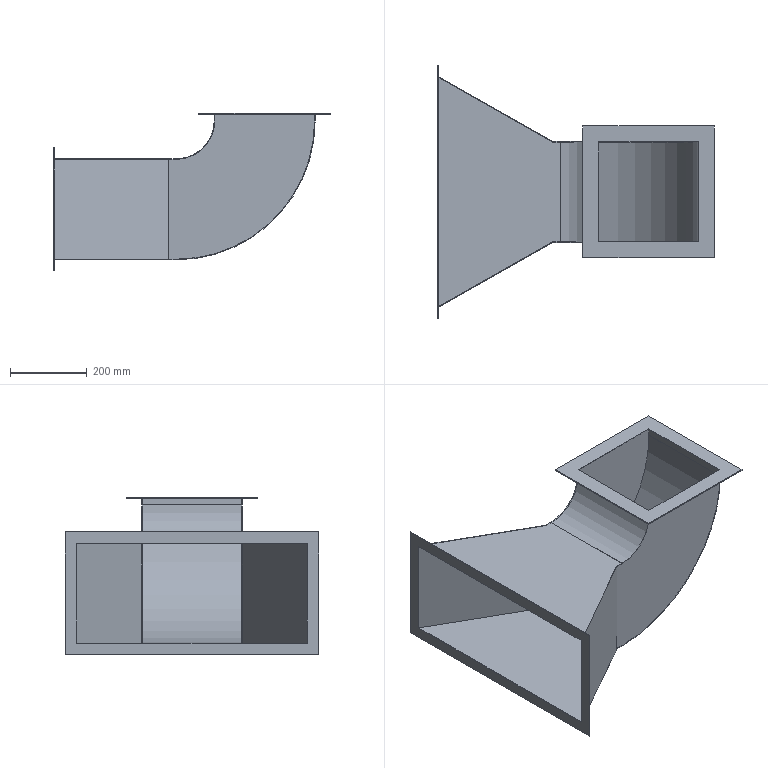Part | STEP file | Produce dryer line heating fan-OVEN-402 | 1 solid | 34 faces | box 721.5 x 660 x 410 mm | volume 1592936 mm3 | plane 30 | cylinder 4 | commonest cylinder face diameters 197 x1 200 x1 720 x1 723 x1
STEP:
#1=CARTESIAN_POINT('',(681.5,131.5,230.));
#2=VERTEX_POINT('',#1);
#3=CARTESIAN_POINT('',(681.5,131.5,247.));
#4=VERTEX_POINT('',#3);
#5=CARTESIAN_POINT('',(681.5,131.5,230.));
#6=DIRECTION('',(0.,0.,1.));
#7=VECTOR('',#6,1000.);
#8=LINE('',#5,#7);
#9=EDGE_CURVE('',#2,#4,#8,.T.);
#10=ORIENTED_EDGE('',*,*,#9,.T.);
#11=CARTESIAN_POINT('',(681.5,-131.5,247.));
#12=VERTEX_POINT('',#11);
#13=CARTESIAN_POINT('',(681.5,131.5,247.));
#14=DIRECTION('',(0.,1.,0.));
#15=VECTOR('',#14,1000.);
#16=LINE('',#13,#15);
#17=EDGE_CURVE('',#12,#4,#16,.T.);
#18=ORIENTED_EDGE('',*,*,#17,.F.);
#19=CARTESIAN_POINT('',(681.5,-131.5,230.));
#20=VERTEX_POINT('',#19);
#21=CARTESIAN_POINT('',(681.5,-131.5,230.));
#22=DIRECTION('',(0.,0.,1.));
#23=VECTOR('',#22,1000.);
#24=LINE('',#21,#23);
#25=EDGE_CURVE('',#20,#12,#24,.T.);
#26=ORIENTED_EDGE('',*,*,#25,.F.);
#27=CARTESIAN_POINT('',(681.5,130.,230.));
#28=DIRECTION('',(0.,1.,0.));
#29=VECTOR('',#28,1000.);
#30=LINE('',#27,#29);
#31=EDGE_CURVE('',#20,#2,#30,.T.);
#32=ORIENTED_EDGE('',*,*,#31,.T.);
#33=EDGE_LOOP('',(#10,#18,#26,#32));
#34=FACE_OUTER_BOUND('',#33,.T.);
#35=CARTESIAN_POINT('',(681.5,130.,230.));
#36=DIRECTION('',(1.,0.,0.));
#37=DIRECTION('',(0.,0.,-1.));
#38=AXIS2_PLACEMENT_3D('',#35,#36,#37);
#39=PLANE('',#38);
#40=ADVANCED_FACE('',(#34),#39,.T.);
#41=CARTESIAN_POINT('',(418.5,-131.5,230.));
#42=VERTEX_POINT('',#41);
#43=CARTESIAN_POINT('',(418.5,-131.5,247.));
#44=VERTEX_POINT('',#43);
#45=CARTESIAN_POINT('',(418.5,-131.5,230.));
#46=DIRECTION('',(0.,0.,1.));
#47=VECTOR('',#46,1000.);
#48=LINE('',#45,#47);
#49=EDGE_CURVE('',#42,#44,#48,.T.);
#50=ORIENTED_EDGE('',*,*,#49,.T.);
#51=CARTESIAN_POINT('',(418.5,131.5,247.));
#52=VERTEX_POINT('',#51);
#53=CARTESIAN_POINT('',(418.5,131.5,247.));
#54=DIRECTION('',(0.,-1.,0.));
#55=VECTOR('',#54,1000.);
#56=LINE('',#53,#55);
#57=EDGE_CURVE('',#52,#44,#56,.T.);
#58=ORIENTED_EDGE('',*,*,#57,.F.);
#59=CARTESIAN_POINT('',(418.5,131.5,230.));
#60=VERTEX_POINT('',#59);
#61=CARTESIAN_POINT('',(418.5,131.5,230.));
#62=DIRECTION('',(0.,0.,1.));
#63=VECTOR('',#62,1000.);
#64=LINE('',#61,#63);
#65=EDGE_CURVE('',#60,#52,#64,.T.);
#66=ORIENTED_EDGE('',*,*,#65,.F.);
#67=CARTESIAN_POINT('',(418.5,130.,230.));
#68=DIRECTION('',(0.,-1.,0.));
#69=VECTOR('',#68,1000.);
#70=LINE('',#67,#69);
#71=EDGE_CURVE('',#60,#42,#70,.T.);
#72=ORIENTED_EDGE('',*,*,#71,.T.);
#73=EDGE_LOOP('',(#50,#58,#66,#72));
#74=FACE_OUTER_BOUND('',#73,.T.);
#75=CARTESIAN_POINT('',(418.5,130.,230.));
#76=DIRECTION('',(-1.,0.,0.));
#77=DIRECTION('',(0.,0.,1.));
#78=AXIS2_PLACEMENT_3D('',#75,#76,#77);
#79=PLANE('',#78);
#80=ADVANCED_FACE('',(#74),#79,.T.);
#81=CARTESIAN_POINT('',(418.5,-131.5,247.));
#82=DIRECTION('',(1.,0.,0.));
#83=VECTOR('',#82,1000.);
#84=LINE('',#81,#83);
#85=EDGE_CURVE('',#44,#12,#84,.T.);
#86=ORIENTED_EDGE('',*,*,#85,.F.);
#87=ORIENTED_EDGE('',*,*,#49,.F.);
#88=CARTESIAN_POINT('',(320.,-131.5,131.5));
#89=VERTEX_POINT('',#88);
#90=CARTESIAN_POINT('',(320.,-131.5,230.));
#91=DIRECTION('',(0.,-1.,0.));
#92=DIRECTION('',(0.,0.,-1.));
#93=AXIS2_PLACEMENT_3D('',#90,#91,#92);
#94=CIRCLE('',#93,98.5);
#95=EDGE_CURVE('',#89,#42,#94,.T.);
#96=ORIENTED_EDGE('',*,*,#95,.F.);
#97=CARTESIAN_POINT('',(300.,-131.5,131.5));
#98=VERTEX_POINT('',#97);
#99=CARTESIAN_POINT('',(320.,-131.5,131.5));
#100=DIRECTION('',(-1.,0.,0.));
#101=VECTOR('',#100,1000.);
#102=LINE('',#99,#101);
#103=EDGE_CURVE('',#89,#98,#102,.T.);
#104=ORIENTED_EDGE('',*,*,#103,.T.);
#105=CARTESIAN_POINT('',(300.,-131.5,-131.5));
#106=VERTEX_POINT('',#105);
#107=CARTESIAN_POINT('',(300.,-131.5,130.));
#108=DIRECTION('',(0.,0.,-1.));
#109=VECTOR('',#108,1000.);
#110=LINE('',#107,#109);
#111=EDGE_CURVE('',#98,#106,#110,.T.);
#112=ORIENTED_EDGE('',*,*,#111,.T.);
#113=CARTESIAN_POINT('',(320.,-131.5,-131.5));
#114=VERTEX_POINT('',#113);
#115=CARTESIAN_POINT('',(320.,-131.5,-131.5));
#116=DIRECTION('',(-1.,0.,0.));
#117=VECTOR('',#116,1000.);
#118=LINE('',#115,#117);
#119=EDGE_CURVE('',#114,#106,#118,.T.);
#120=ORIENTED_EDGE('',*,*,#119,.F.);
#121=CARTESIAN_POINT('',(320.,-131.5,230.));
#122=DIRECTION('',(0.,-1.,0.));
#123=DIRECTION('',(0.,0.,-1.));
#124=AXIS2_PLACEMENT_3D('',#121,#122,#123);
#125=CIRCLE('',#124,361.5);
#126=EDGE_CURVE('',#114,#20,#125,.T.);
#127=ORIENTED_EDGE('',*,*,#126,.T.);
#128=ORIENTED_EDGE('',*,*,#25,.T.);
#129=EDGE_LOOP('',(#86,#87,#96,#104,#112,#120,#127,#128));
#130=FACE_OUTER_BOUND('',#129,.T.);
#131=CARTESIAN_POINT('',(320.,-131.5,130.));
#132=DIRECTION('',(0.,1.,0.));
#133=DIRECTION('',(0.,0.,1.));
#134=AXIS2_PLACEMENT_3D('',#131,#132,#133);
#135=PLANE('',#134);
#136=ADVANCED_FACE('',(#130),#135,.F.);
#137=CARTESIAN_POINT('',(418.5,131.5,247.));
#138=DIRECTION('',(-1.,0.,0.));
#139=VECTOR('',#138,1000.);
#140=LINE('',#137,#139);
#141=EDGE_CURVE('',#4,#52,#140,.T.);
#142=ORIENTED_EDGE('',*,*,#141,.F.);
#143=ORIENTED_EDGE('',*,*,#9,.F.);
#144=CARTESIAN_POINT('',(320.,131.5,-131.5));
#145=VERTEX_POINT('',#144);
#146=CARTESIAN_POINT('',(320.,131.5,230.));
#147=DIRECTION('',(0.,-1.,0.));
#148=DIRECTION('',(0.,0.,1.));
#149=AXIS2_PLACEMENT_3D('',#146,#147,#148);
#150=CIRCLE('',#149,361.5);
#151=EDGE_CURVE('',#145,#2,#150,.T.);
#152=ORIENTED_EDGE('',*,*,#151,.F.);
#153=CARTESIAN_POINT('',(300.,131.5,-131.5));
#154=VERTEX_POINT('',#153);
#155=CARTESIAN_POINT('',(320.,131.5,-131.5));
#156=DIRECTION('',(-1.,0.,0.));
#157=VECTOR('',#156,1000.);
#158=LINE('',#155,#157);
#159=EDGE_CURVE('',#145,#154,#158,.T.);
#160=ORIENTED_EDGE('',*,*,#159,.T.);
#161=CARTESIAN_POINT('',(300.,131.5,131.5));
#162=VERTEX_POINT('',#161);
#163=CARTESIAN_POINT('',(300.,131.5,130.));
#164=DIRECTION('',(0.,0.,1.));
#165=VECTOR('',#164,1000.);
#166=LINE('',#163,#165);
#167=EDGE_CURVE('',#154,#162,#166,.T.);
#168=ORIENTED_EDGE('',*,*,#167,.T.);
#169=CARTESIAN_POINT('',(320.,131.5,131.5));
#170=VERTEX_POINT('',#169);
#171=CARTESIAN_POINT('',(320.,131.5,131.5));
#172=DIRECTION('',(-1.,0.,0.));
#173=VECTOR('',#172,1000.);
#174=LINE('',#171,#173);
#175=EDGE_CURVE('',#170,#162,#174,.T.);
#176=ORIENTED_EDGE('',*,*,#175,.F.);
#177=CARTESIAN_POINT('',(320.,131.5,230.));
#178=DIRECTION('',(0.,-1.,0.));
#179=DIRECTION('',(0.,0.,1.));
#180=AXIS2_PLACEMENT_3D('',#177,#178,#179);
#181=CIRCLE('',#180,98.5);
#182=EDGE_CURVE('',#170,#60,#181,.T.);
#183=ORIENTED_EDGE('',*,*,#182,.T.);
#184=ORIENTED_EDGE('',*,*,#65,.T.);
#185=EDGE_LOOP('',(#142,#143,#152,#160,#168,#176,#183,#184));
#186=FACE_OUTER_BOUND('',#185,.T.);
#187=CARTESIAN_POINT('',(320.,131.5,130.));
#188=DIRECTION('',(0.,-1.,0.));
#189=DIRECTION('',(0.,0.,-1.));
#190=AXIS2_PLACEMENT_3D('',#187,#188,#189);
#191=PLANE('',#190);
#192=ADVANCED_FACE('',(#186),#191,.F.);
#193=ORIENTED_EDGE('',*,*,#167,.F.);
#194=CARTESIAN_POINT('',(300.,131.724,-131.5));
#195=VERTEX_POINT('',#194);
#196=CARTESIAN_POINT('',(300.,130.,-131.5));
#197=DIRECTION('',(0.,1.,0.));
#198=VECTOR('',#197,1000.);
#199=LINE('',#196,#198);
#200=EDGE_CURVE('',#154,#195,#199,.T.);
#201=ORIENTED_EDGE('',*,*,#200,.T.);
#202=CARTESIAN_POINT('',(300.,131.724,131.5));
#203=VERTEX_POINT('',#202);
#204=CARTESIAN_POINT('',(300.,131.724,130.));
#205=DIRECTION('',(0.,0.,1.));
#206=VECTOR('',#205,1000.);
#207=LINE('',#204,#206);
#208=EDGE_CURVE('',#195,#203,#207,.T.);
#209=ORIENTED_EDGE('',*,*,#208,.T.);
#210=CARTESIAN_POINT('',(300.,-130.,131.5));
#211=DIRECTION('',(0.,-1.,0.));
#212=VECTOR('',#211,1000.);
#213=LINE('',#210,#212);
#214=EDGE_CURVE('',#203,#162,#213,.T.);
#215=ORIENTED_EDGE('',*,*,#214,.T.);
#216=EDGE_LOOP('',(#193,#201,#209,#215));
#217=FACE_OUTER_BOUND('',#216,.T.);
#218=CARTESIAN_POINT('',(300.,-130.,130.));
#219=DIRECTION('',(1.,0.,0.));
#220=DIRECTION('',(0.,0.,-1.));
#221=AXIS2_PLACEMENT_3D('',#218,#219,#220);
#222=PLANE('',#221);
#223=ADVANCED_FACE('',(#217),#222,.T.);
#224=CARTESIAN_POINT('',(3.,330.,160.));
#225=VERTEX_POINT('',#224);
#226=CARTESIAN_POINT('',(3.,-330.,160.));
#227=VERTEX_POINT('',#226);
#228=CARTESIAN_POINT('',(3.,330.,160.));
#229=DIRECTION('',(0.,-1.,0.));
#230=VECTOR('',#229,1000.);
#231=LINE('',#228,#230);
#232=EDGE_CURVE('',#225,#227,#231,.T.);
#233=ORIENTED_EDGE('',*,*,#232,.T.);
#234=CARTESIAN_POINT('',(3.,-330.,-160.));
#235=VERTEX_POINT('',#234);
#236=CARTESIAN_POINT('',(3.,-330.,160.));
#237=DIRECTION('',(0.,0.,-1.));
#238=VECTOR('',#237,1000.);
#239=LINE('',#236,#238);
#240=EDGE_CURVE('',#227,#235,#239,.T.);
#241=ORIENTED_EDGE('',*,*,#240,.T.);
#242=CARTESIAN_POINT('',(3.,330.,-160.));
#243=VERTEX_POINT('',#242);
#244=CARTESIAN_POINT('',(3.,330.,-160.));
#245=DIRECTION('',(0.,1.,0.));
#246=VECTOR('',#245,1000.);
#247=LINE('',#244,#246);
#248=EDGE_CURVE('',#235,#243,#247,.T.);
#249=ORIENTED_EDGE('',*,*,#248,.T.);
#250=CARTESIAN_POINT('',(3.,330.,160.));
#251=DIRECTION('',(0.,0.,1.));
#252=VECTOR('',#251,1000.);
#253=LINE('',#250,#252);
#254=EDGE_CURVE('',#243,#225,#253,.T.);
#255=ORIENTED_EDGE('',*,*,#254,.T.);
#256=EDGE_LOOP('',(#233,#241,#249,#255));
#257=FACE_OUTER_BOUND('',#256,.T.);
#258=CARTESIAN_POINT('',(3.,300.024,-131.5));
#259=VERTEX_POINT('',#258);
#260=CARTESIAN_POINT('',(3.,-300.024,-131.5));
#261=VERTEX_POINT('',#260);
#262=CARTESIAN_POINT('',(3.,-330.,-131.5));
#263=DIRECTION('',(0.,-1.,0.));
#264=VECTOR('',#263,1000.);
#265=LINE('',#262,#264);
#266=EDGE_CURVE('',#259,#261,#265,.T.);
#267=ORIENTED_EDGE('',*,*,#266,.T.);
#268=CARTESIAN_POINT('',(3.,-300.024,131.5));
#269=VERTEX_POINT('',#268);
#270=CARTESIAN_POINT('',(3.,-300.024,160.));
#271=DIRECTION('',(0.,0.,1.));
#272=VECTOR('',#271,1000.);
#273=LINE('',#270,#272);
#274=EDGE_CURVE('',#261,#269,#273,.T.);
#275=ORIENTED_EDGE('',*,*,#274,.T.);
#276=CARTESIAN_POINT('',(3.,300.024,131.5));
#277=VERTEX_POINT('',#276);
#278=CARTESIAN_POINT('',(3.,-330.,131.5));
#279=DIRECTION('',(0.,1.,0.));
#280=VECTOR('',#279,1000.);
#281=LINE('',#278,#280);
#282=EDGE_CURVE('',#269,#277,#281,.T.);
#283=ORIENTED_EDGE('',*,*,#282,.T.);
#284=CARTESIAN_POINT('',(3.,300.024,160.));
#285=DIRECTION('',(0.,0.,-1.));
#286=VECTOR('',#285,1000.);
#287=LINE('',#284,#286);
#288=EDGE_CURVE('',#277,#259,#287,.T.);
#289=ORIENTED_EDGE('',*,*,#288,.T.);
#290=EDGE_LOOP('',(#267,#275,#283,#289));
#291=FACE_BOUND('',#290,.T.);
#292=CARTESIAN_POINT('',(3.,-330.,160.));
#293=DIRECTION('',(1.,0.,0.));
#294=DIRECTION('',(0.,0.,-1.));
#295=AXIS2_PLACEMENT_3D('',#292,#293,#294);
#296=PLANE('',#295);
#297=ADVANCED_FACE('',(#257,#291),#296,.T.);
#298=CARTESIAN_POINT('',(0.,300.,130.));
#299=VERTEX_POINT('',#298);
#300=CARTESIAN_POINT('',(0.,-300.,130.));
#301=VERTEX_POINT('',#300);
#302=CARTESIAN_POINT('',(0.,300.,130.));
#303=DIRECTION('',(0.,-1.,0.));
#304=VECTOR('',#303,1000.);
#305=LINE('',#302,#304);
#306=EDGE_CURVE('',#299,#301,#305,.T.);
#307=ORIENTED_EDGE('',*,*,#306,.T.);
#308=CARTESIAN_POINT('',(0.,-300.,-130.));
#309=VERTEX_POINT('',#308);
#310=CARTESIAN_POINT('',(0.,-300.,130.));
#311=CARTESIAN_POINT('',(0.,-300.,43.333));
#312=CARTESIAN_POINT('',(0.,-300.,-43.333));
#313=CARTESIAN_POINT('',(0.,-300.,-130.));
#314=B_SPLINE_CURVE_WITH_KNOTS('',3,(#310,#311,#312,#313),.UNSPECIFIED.,.F.,.F.,(4,4),(0.,1.),.UNSPECIFIED.);
#315=EDGE_CURVE('',#301,#309,#314,.T.);
#316=ORIENTED_EDGE('',*,*,#315,.T.);
#317=CARTESIAN_POINT('',(0.,300.,-130.));
#318=VERTEX_POINT('',#317);
#319=CARTESIAN_POINT('',(0.,300.,-130.));
#320=DIRECTION('',(0.,1.,0.));
#321=VECTOR('',#320,1000.);
#322=LINE('',#319,#321);
#323=EDGE_CURVE('',#309,#318,#322,.T.);
#324=ORIENTED_EDGE('',*,*,#323,.T.);
#325=CARTESIAN_POINT('',(0.,300.,-130.));
#326=CARTESIAN_POINT('',(0.,300.,-43.333));
#327=CARTESIAN_POINT('',(0.,300.,43.333));
#328=CARTESIAN_POINT('',(0.,300.,130.));
#329=B_SPLINE_CURVE_WITH_KNOTS('',3,(#325,#326,#327,#328),.UNSPECIFIED.,.F.,.F.,(4,4),(0.,1.),.UNSPECIFIED.);
#330=EDGE_CURVE('',#318,#299,#329,.T.);
#331=ORIENTED_EDGE('',*,*,#330,.T.);
#332=EDGE_LOOP('',(#307,#316,#324,#331));
#333=FACE_BOUND('',#332,.T.);
#334=CARTESIAN_POINT('',(0.,330.,160.));
#335=VERTEX_POINT('',#334);
#336=CARTESIAN_POINT('',(0.,-330.,160.));
#337=VERTEX_POINT('',#336);
#338=CARTESIAN_POINT('',(0.,330.,160.));
#339=DIRECTION('',(0.,-1.,0.));
#340=VECTOR('',#339,1000.);
#341=LINE('',#338,#340);
#342=EDGE_CURVE('',#335,#337,#341,.T.);
#343=ORIENTED_EDGE('',*,*,#342,.F.);
#344=CARTESIAN_POINT('',(0.,330.,-160.));
#345=VERTEX_POINT('',#344);
#346=CARTESIAN_POINT('',(0.,330.,160.));
#347=DIRECTION('',(0.,0.,1.));
#348=VECTOR('',#347,1000.);
#349=LINE('',#346,#348);
#350=EDGE_CURVE('',#345,#335,#349,.T.);
#351=ORIENTED_EDGE('',*,*,#350,.F.);
#352=CARTESIAN_POINT('',(0.,-330.,-160.));
#353=VERTEX_POINT('',#352);
#354=CARTESIAN_POINT('',(0.,330.,-160.));
#355=DIRECTION('',(0.,1.,0.));
#356=VECTOR('',#355,1000.);
#357=LINE('',#354,#356);
#358=EDGE_CURVE('',#353,#345,#357,.T.);
#359=ORIENTED_EDGE('',*,*,#358,.F.);
#360=CARTESIAN_POINT('',(0.,-330.,160.));
#361=DIRECTION('',(0.,0.,-1.));
#362=VECTOR('',#361,1000.);
#363=LINE('',#360,#362);
#364=EDGE_CURVE('',#337,#353,#363,.T.);
#365=ORIENTED_EDGE('',*,*,#364,.F.);
#366=EDGE_LOOP('',(#343,#351,#359,#365));
#367=FACE_OUTER_BOUND('',#366,.T.);
#368=CARTESIAN_POINT('',(0.,-330.,160.));
#369=DIRECTION('',(1.,0.,0.));
#370=DIRECTION('',(0.,0.,-1.));
#371=AXIS2_PLACEMENT_3D('',#368,#369,#370);
#372=PLANE('',#371);
#373=ADVANCED_FACE('',(#333,#367),#372,.F.);
#374=ORIENTED_EDGE('',*,*,#342,.T.);
#375=CARTESIAN_POINT('',(3.,-330.,160.));
#376=DIRECTION('',(-1.,0.,0.));
#377=VECTOR('',#376,1000.);
#378=LINE('',#375,#377);
#379=EDGE_CURVE('',#227,#337,#378,.T.);
#380=ORIENTED_EDGE('',*,*,#379,.F.);
#381=ORIENTED_EDGE('',*,*,#232,.F.);
#382=CARTESIAN_POINT('',(3.,330.,160.));
#383=DIRECTION('',(-1.,0.,0.));
#384=VECTOR('',#383,1000.);
#385=LINE('',#382,#384);
#386=EDGE_CURVE('',#225,#335,#385,.T.);
#387=ORIENTED_EDGE('',*,*,#386,.T.);
#388=EDGE_LOOP('',(#374,#380,#381,#387));
#389=FACE_OUTER_BOUND('',#388,.T.);
#390=CARTESIAN_POINT('',(3.,330.,160.));
#391=DIRECTION('',(0.,0.,-1.));
#392=DIRECTION('',(0.,1.,0.));
#393=AXIS2_PLACEMENT_3D('',#390,#391,#392);
#394=PLANE('',#393);
#395=ADVANCED_FACE('',(#389),#394,.F.);
#396=ORIENTED_EDGE('',*,*,#364,.T.);
#397=CARTESIAN_POINT('',(3.,-330.,-160.));
#398=DIRECTION('',(-1.,0.,0.));
#399=VECTOR('',#398,1000.);
#400=LINE('',#397,#399);
#401=EDGE_CURVE('',#235,#353,#400,.T.);
#402=ORIENTED_EDGE('',*,*,#401,.F.);
#403=ORIENTED_EDGE('',*,*,#240,.F.);
#404=ORIENTED_EDGE('',*,*,#379,.T.);
#405=EDGE_LOOP('',(#396,#402,#403,#404));
#406=FACE_OUTER_BOUND('',#405,.T.);
#407=CARTESIAN_POINT('',(3.,-330.,160.));
#408=DIRECTION('',(0.,1.,0.));
#409=DIRECTION('',(0.,0.,1.));
#410=AXIS2_PLACEMENT_3D('',#407,#408,#409);
#411=PLANE('',#410);
#412=ADVANCED_FACE('',(#406),#411,.F.);
#413=ORIENTED_EDGE('',*,*,#358,.T.);
#414=CARTESIAN_POINT('',(3.,330.,-160.));
#415=DIRECTION('',(-1.,0.,0.));
#416=VECTOR('',#415,1000.);
#417=LINE('',#414,#416);
#418=EDGE_CURVE('',#243,#345,#417,.T.);
#419=ORIENTED_EDGE('',*,*,#418,.F.);
#420=ORIENTED_EDGE('',*,*,#248,.F.);
#421=ORIENTED_EDGE('',*,*,#401,.T.);
#422=EDGE_LOOP('',(#413,#419,#420,#421));
#423=FACE_OUTER_BOUND('',#422,.T.);
#424=CARTESIAN_POINT('',(3.,330.,-160.));
#425=DIRECTION('',(0.,0.,1.));
#426=DIRECTION('',(0.,-1.,0.));
#427=AXIS2_PLACEMENT_3D('',#424,#425,#426);
#428=PLANE('',#427);
#429=ADVANCED_FACE('',(#423),#428,.F.);
#430=ORIENTED_EDGE('',*,*,#350,.T.);
#431=ORIENTED_EDGE('',*,*,#386,.F.);
#432=ORIENTED_EDGE('',*,*,#254,.F.);
#433=ORIENTED_EDGE('',*,*,#418,.T.);
#434=EDGE_LOOP('',(#430,#431,#432,#433));
#435=FACE_OUTER_BOUND('',#434,.T.);
#436=CARTESIAN_POINT('',(3.,330.,160.));
#437=DIRECTION('',(0.,-1.,0.));
#438=DIRECTION('',(0.,0.,-1.));
#439=AXIS2_PLACEMENT_3D('',#436,#437,#438);
#440=PLANE('',#439);
#441=ADVANCED_FACE('',(#435),#440,.F.);
#442=CARTESIAN_POINT('',(300.,-130.,130.));
#443=VERTEX_POINT('',#442);
#444=CARTESIAN_POINT('',(0.,-300.,130.));
#445=DIRECTION('',(0.87,0.493,0.));
#446=VECTOR('',#445,1000.);
#447=LINE('',#444,#446);
#448=EDGE_CURVE('',#301,#443,#447,.T.);
#449=ORIENTED_EDGE('',*,*,#448,.F.);
#450=ORIENTED_EDGE('',*,*,#306,.F.);
#451=CARTESIAN_POINT('',(300.,130.,130.));
#452=VERTEX_POINT('',#451);
#453=CARTESIAN_POINT('',(0.,300.,130.));
#454=DIRECTION('',(0.87,-0.493,0.));
#455=VECTOR('',#454,1000.);
#456=LINE('',#453,#455);
#457=EDGE_CURVE('',#299,#452,#456,.T.);
#458=ORIENTED_EDGE('',*,*,#457,.T.);
#459=CARTESIAN_POINT('',(320.,130.,130.));
#460=VERTEX_POINT('',#459);
#461=CARTESIAN_POINT('',(320.,130.,130.));
#462=DIRECTION('',(-1.,0.,0.));
#463=VECTOR('',#462,1000.);
#464=LINE('',#461,#463);
#465=EDGE_CURVE('',#460,#452,#464,.T.);
#466=ORIENTED_EDGE('',*,*,#465,.F.);
#467=CARTESIAN_POINT('',(320.,-130.,130.));
#468=VERTEX_POINT('',#467);
#469=CARTESIAN_POINT('',(320.,130.,130.));
#470=DIRECTION('',(0.,-1.,0.));
#471=VECTOR('',#470,1000.);
#472=LINE('',#469,#471);
#473=EDGE_CURVE('',#460,#468,#472,.T.);
#474=ORIENTED_EDGE('',*,*,#473,.T.);
#475=CARTESIAN_POINT('',(320.,-130.,130.));
#476=DIRECTION('',(-1.,0.,0.));
#477=VECTOR('',#476,1000.);
#478=LINE('',#475,#477);
#479=EDGE_CURVE('',#468,#443,#478,.T.);
#480=ORIENTED_EDGE('',*,*,#479,.T.);
#481=EDGE_LOOP('',(#449,#450,#458,#466,#474,#480));
#482=FACE_OUTER_BOUND('',#481,.T.);
#483=CARTESIAN_POINT('',(3.,300.,130.));
#484=DIRECTION('',(0.,0.,-1.));
#485=DIRECTION('',(-1.,0.,0.));
#486=AXIS2_PLACEMENT_3D('',#483,#484,#485);
#487=PLANE('',#486);
#488=ADVANCED_FACE('',(#482),#487,.T.);
#489=CARTESIAN_POINT('',(300.,-130.,-130.));
#490=VERTEX_POINT('',#489);
#491=CARTESIAN_POINT('',(0.,-300.,-130.));
#492=DIRECTION('',(0.87,0.493,0.));
#493=VECTOR('',#492,1000.);
#494=LINE('',#491,#493);
#495=EDGE_CURVE('',#309,#490,#494,.T.);
#496=ORIENTED_EDGE('',*,*,#495,.T.);
#497=CARTESIAN_POINT('',(320.,-130.,-130.));
#498=VERTEX_POINT('',#497);
#499=CARTESIAN_POINT('',(320.,-130.,-130.));
#500=DIRECTION('',(-1.,0.,0.));
#501=VECTOR('',#500,1000.);
#502=LINE('',#499,#501);
#503=EDGE_CURVE('',#498,#490,#502,.T.);
#504=ORIENTED_EDGE('',*,*,#503,.F.);
#505=CARTESIAN_POINT('',(320.,130.,-130.));
#506=VERTEX_POINT('',#505);
#507=CARTESIAN_POINT('',(320.,130.,-130.));
#508=DIRECTION('',(0.,1.,0.));
#509=VECTOR('',#508,1000.);
#510=LINE('',#507,#509);
#511=EDGE_CURVE('',#498,#506,#510,.T.);
#512=ORIENTED_EDGE('',*,*,#511,.T.);
#513=CARTESIAN_POINT('',(300.,130.,-130.));
#514=VERTEX_POINT('',#513);
#515=CARTESIAN_POINT('',(320.,130.,-130.));
#516=DIRECTION('',(-1.,0.,0.));
#517=VECTOR('',#516,1000.);
#518=LINE('',#515,#517);
#519=EDGE_CURVE('',#506,#514,#518,.T.);
#520=ORIENTED_EDGE('',*,*,#519,.T.);
#521=CARTESIAN_POINT('',(0.,300.,-130.));
#522=DIRECTION('',(0.87,-0.493,0.));
#523=VECTOR('',#522,1000.);
#524=LINE('',#521,#523);
#525=EDGE_CURVE('',#318,#514,#524,.T.);
#526=ORIENTED_EDGE('',*,*,#525,.F.);
#527=ORIENTED_EDGE('',*,*,#323,.F.);
#528=EDGE_LOOP('',(#496,#504,#512,#520,#526,#527));
#529=FACE_OUTER_BOUND('',#528,.T.);
#530=CARTESIAN_POINT('',(3.,300.,-130.));
#531=DIRECTION('',(0.,0.,1.));
#532=DIRECTION('',(0.,-1.,0.));
#533=AXIS2_PLACEMENT_3D('',#530,#531,#532);
#534=PLANE('',#533);
#535=ADVANCED_FACE('',(#529),#534,.T.);
#536=ORIENTED_EDGE('',*,*,#111,.F.);
#537=CARTESIAN_POINT('',(300.,-131.724,131.5));
#538=VERTEX_POINT('',#537);
#539=CARTESIAN_POINT('',(300.,-130.,131.5));
#540=DIRECTION('',(0.,-1.,0.));
#541=VECTOR('',#540,1000.);
#542=LINE('',#539,#541);
#543=EDGE_CURVE('',#98,#538,#542,.T.);
#544=ORIENTED_EDGE('',*,*,#543,.T.);
#545=CARTESIAN_POINT('',(300.,-131.724,-131.5));
#546=VERTEX_POINT('',#545);
#547=CARTESIAN_POINT('',(300.,-131.724,-130.));
#548=DIRECTION('',(0.,0.,-1.));
#549=VECTOR('',#548,1000.);
#550=LINE('',#547,#549);
#551=EDGE_CURVE('',#538,#546,#550,.T.);
#552=ORIENTED_EDGE('',*,*,#551,.T.);
#553=CARTESIAN_POINT('',(300.,130.,-131.5));
#554=DIRECTION('',(0.,1.,0.));
#555=VECTOR('',#554,1000.);
#556=LINE('',#553,#555);
#557=EDGE_CURVE('',#546,#106,#556,.T.);
#558=ORIENTED_EDGE('',*,*,#557,.T.);
#559=EDGE_LOOP('',(#536,#544,#552,#558));
#560=FACE_OUTER_BOUND('',#559,.T.);
#561=CARTESIAN_POINT('',(300.,-130.,130.));
#562=DIRECTION('',(1.,0.,0.));
#563=DIRECTION('',(0.,0.,-1.));
#564=AXIS2_PLACEMENT_3D('',#561,#562,#563);
#565=PLANE('',#564);
#566=ADVANCED_FACE('',(#560),#565,.T.);
#567=ORIENTED_EDGE('',*,*,#274,.F.);
#568=CARTESIAN_POINT('',(300.74,-131.305,-131.5));
#569=DIRECTION('',(0.87,0.493,0.));
#570=VECTOR('',#569,1000.);
#571=LINE('',#568,#570);
#572=EDGE_CURVE('',#261,#546,#571,.T.);
#573=ORIENTED_EDGE('',*,*,#572,.T.);
#574=ORIENTED_EDGE('',*,*,#551,.F.);
#575=CARTESIAN_POINT('',(300.74,-131.305,131.5));
#576=DIRECTION('',(0.87,0.493,0.));
#577=VECTOR('',#576,1000.);
#578=LINE('',#575,#577);
#579=EDGE_CURVE('',#269,#538,#578,.T.);
#580=ORIENTED_EDGE('',*,*,#579,.F.);
#581=EDGE_LOOP('',(#567,#573,#574,#580));
#582=FACE_OUTER_BOUND('',#581,.T.);
#583=CARTESIAN_POINT('',(300.74,-131.305,-130.));
#584=DIRECTION('',(-0.493,0.87,0.));
#585=DIRECTION('',(-0.87,-0.493,0.));
#586=AXIS2_PLACEMENT_3D('',#583,#584,#585);
#587=PLANE('',#586);
#588=ADVANCED_FACE('',(#582),#587,.F.);
#589=ORIENTED_EDGE('',*,*,#282,.F.);
#590=ORIENTED_EDGE('',*,*,#579,.T.);
#591=ORIENTED_EDGE('',*,*,#543,.F.);
#592=ORIENTED_EDGE('',*,*,#103,.F.);
#593=CARTESIAN_POINT('',(320.,0.,131.5));
#594=DIRECTION('',(0.,-1.,0.));
#595=VECTOR('',#594,1000.);
#596=LINE('',#593,#595);
#597=EDGE_CURVE('',#170,#89,#596,.T.);
#598=ORIENTED_EDGE('',*,*,#597,.F.);
#599=ORIENTED_EDGE('',*,*,#175,.T.);
#600=ORIENTED_EDGE('',*,*,#214,.F.);
#601=CARTESIAN_POINT('',(300.74,131.305,131.5));
#602=DIRECTION('',(0.87,-0.493,0.));
#603=VECTOR('',#602,1000.);
#604=LINE('',#601,#603);
#605=EDGE_CURVE('',#277,#203,#604,.T.);
#606=ORIENTED_EDGE('',*,*,#605,.F.);
#607=EDGE_LOOP('',(#589,#590,#591,#592,#598,#599,#600,#606));
#608=FACE_OUTER_BOUND('',#607,.T.);
#609=CARTESIAN_POINT('',(300.,-130.,131.5));
#610=DIRECTION('',(0.,0.,-1.));
#611=DIRECTION('',(-1.,0.,0.));
#612=AXIS2_PLACEMENT_3D('',#609,#610,#611);
#613=PLANE('',#612);
#614=ADVANCED_FACE('',(#608),#613,.F.);
#615=ORIENTED_EDGE('',*,*,#266,.F.);
#616=CARTESIAN_POINT('',(300.74,131.305,-131.5));
#617=DIRECTION('',(0.87,-0.493,0.));
#618=VECTOR('',#617,1000.);
#619=LINE('',#616,#618);
#620=EDGE_CURVE('',#259,#195,#619,.T.);
#621=ORIENTED_EDGE('',*,*,#620,.T.);
#622=ORIENTED_EDGE('',*,*,#200,.F.);
#623=ORIENTED_EDGE('',*,*,#159,.F.);
#624=CARTESIAN_POINT('',(320.,0.,-131.5));
#625=DIRECTION('',(0.,1.,0.));
#626=VECTOR('',#625,1000.);
#627=LINE('',#624,#626);
#628=EDGE_CURVE('',#114,#145,#627,.T.);
#629=ORIENTED_EDGE('',*,*,#628,.F.);
#630=ORIENTED_EDGE('',*,*,#119,.T.);
#631=ORIENTED_EDGE('',*,*,#557,.F.);
#632=ORIENTED_EDGE('',*,*,#572,.F.);
#633=EDGE_LOOP('',(#615,#621,#622,#623,#629,#630,#631,#632));
#634=FACE_OUTER_BOUND('',#633,.T.);
#635=CARTESIAN_POINT('',(300.,130.,-131.5));
#636=DIRECTION('',(0.,0.,1.));
#637=DIRECTION('',(1.,0.,0.));
#638=AXIS2_PLACEMENT_3D('',#635,#636,#637);
#639=PLANE('',#638);
#640=ADVANCED_FACE('',(#634),#639,.F.);
#641=ORIENTED_EDGE('',*,*,#288,.F.);
#642=ORIENTED_EDGE('',*,*,#605,.T.);
#643=ORIENTED_EDGE('',*,*,#208,.F.);
#644=ORIENTED_EDGE('',*,*,#620,.F.);
#645=EDGE_LOOP('',(#641,#642,#643,#644));
#646=FACE_OUTER_BOUND('',#645,.T.);
#647=CARTESIAN_POINT('',(300.74,131.305,130.));
#648=DIRECTION('',(-0.493,-0.87,0.));
#649=DIRECTION('',(0.87,-0.493,0.));
#650=AXIS2_PLACEMENT_3D('',#647,#648,#649);
#651=PLANE('',#650);
#652=ADVANCED_FACE('',(#646),#651,.F.);
#653=ORIENTED_EDGE('',*,*,#495,.F.);
#654=ORIENTED_EDGE('',*,*,#315,.F.);
#655=ORIENTED_EDGE('',*,*,#448,.T.);
#656=CARTESIAN_POINT('',(300.,-130.,130.));
#657=DIRECTION('',(0.,0.,-1.));
#658=VECTOR('',#657,1000.);
#659=LINE('',#656,#658);
#660=EDGE_CURVE('',#443,#490,#659,.T.);
#661=ORIENTED_EDGE('',*,*,#660,.T.);
#662=EDGE_LOOP('',(#653,#654,#655,#661));
#663=FACE_OUTER_BOUND('',#662,.T.);
#664=CARTESIAN_POINT('',(300.,-130.,-130.));
#665=DIRECTION('',(-0.493,0.87,0.));
#666=DIRECTION('',(-0.87,-0.493,0.));
#667=AXIS2_PLACEMENT_3D('',#664,#665,#666);
#668=PLANE('',#667);
#669=ADVANCED_FACE('',(#663),#668,.T.);
#670=ORIENTED_EDGE('',*,*,#457,.F.);
#671=ORIENTED_EDGE('',*,*,#330,.F.);
#672=ORIENTED_EDGE('',*,*,#525,.T.);
#673=CARTESIAN_POINT('',(300.,130.,130.));
#674=DIRECTION('',(0.,0.,1.));
#675=VECTOR('',#674,1000.);
#676=LINE('',#673,#675);
#677=EDGE_CURVE('',#514,#452,#676,.T.);
#678=ORIENTED_EDGE('',*,*,#677,.T.);
#679=EDGE_LOOP('',(#670,#671,#672,#678));
#680=FACE_OUTER_BOUND('',#679,.T.);
#681=CARTESIAN_POINT('',(300.,130.,130.));
#682=DIRECTION('',(-0.493,-0.87,0.));
#683=DIRECTION('',(0.87,-0.493,0.));
#684=AXIS2_PLACEMENT_3D('',#681,#682,#683);
#685=PLANE('',#684);
#686=ADVANCED_FACE('',(#680),#685,.T.);
#687=ORIENTED_EDGE('',*,*,#628,.T.);
#688=ORIENTED_EDGE('',*,*,#151,.T.);
#689=ORIENTED_EDGE('',*,*,#31,.F.);
#690=ORIENTED_EDGE('',*,*,#126,.F.);
#691=EDGE_LOOP('',(#687,#688,#689,#690));
#692=FACE_OUTER_BOUND('',#691,.T.);
#693=CARTESIAN_POINT('',(320.,0.,230.));
#694=DIRECTION('',(0.,-1.,0.));
#695=DIRECTION('',(0.,0.,-1.));
#696=AXIS2_PLACEMENT_3D('',#693,#694,#695);
#697=CYLINDRICAL_SURFACE('',#696,361.5);
#698=ADVANCED_FACE('',(#692),#697,.T.);
#699=ORIENTED_EDGE('',*,*,#597,.T.);
#700=ORIENTED_EDGE('',*,*,#95,.T.);
#701=ORIENTED_EDGE('',*,*,#71,.F.);
#702=ORIENTED_EDGE('',*,*,#182,.F.);
#703=EDGE_LOOP('',(#699,#700,#701,#702));
#704=FACE_OUTER_BOUND('',#703,.T.);
#705=CARTESIAN_POINT('',(320.,0.,230.));
#706=DIRECTION('',(0.,-1.,0.));
#707=DIRECTION('',(0.,0.,-1.));
#708=AXIS2_PLACEMENT_3D('',#705,#706,#707);
#709=CYLINDRICAL_SURFACE('',#708,98.5);
#710=ADVANCED_FACE('',(#704),#709,.F.);
#711=CARTESIAN_POINT('',(420.,130.,250.));
#712=VERTEX_POINT('',#711);
#713=CARTESIAN_POINT('',(420.,-130.,250.));
#714=VERTEX_POINT('',#713);
#715=CARTESIAN_POINT('',(420.,130.,250.));
#716=DIRECTION('',(0.,-1.,0.));
#717=VECTOR('',#716,1000.);
#718=LINE('',#715,#717);
#719=EDGE_CURVE('',#712,#714,#718,.T.);
#720=ORIENTED_EDGE('',*,*,#719,.F.);
#721=CARTESIAN_POINT('',(680.,130.,250.));
#722=VERTEX_POINT('',#721);
#723=CARTESIAN_POINT('',(420.,130.,250.));
#724=DIRECTION('',(-1.,0.,0.));
#725=VECTOR('',#724,1000.);
#726=LINE('',#723,#725);
#727=EDGE_CURVE('',#722,#712,#726,.T.);
#728=ORIENTED_EDGE('',*,*,#727,.F.);
#729=CARTESIAN_POINT('',(680.,-130.,250.));
#730=VERTEX_POINT('',#729);
#731=CARTESIAN_POINT('',(680.,130.,250.));
#732=DIRECTION('',(0.,1.,0.));
#733=VECTOR('',#732,1000.);
#734=LINE('',#731,#733);
#735=EDGE_CURVE('',#730,#722,#734,.T.);
#736=ORIENTED_EDGE('',*,*,#735,.F.);
#737=CARTESIAN_POINT('',(420.,-130.,250.));
#738=DIRECTION('',(1.,0.,0.));
#739=VECTOR('',#738,1000.);
#740=LINE('',#737,#739);
#741=EDGE_CURVE('',#714,#730,#740,.T.);
#742=ORIENTED_EDGE('',*,*,#741,.F.);
#743=EDGE_LOOP('',(#720,#728,#736,#742));
#744=FACE_BOUND('',#743,.T.);
#745=CARTESIAN_POINT('',(378.5,171.5,250.));
#746=VERTEX_POINT('',#745);
#747=CARTESIAN_POINT('',(378.5,-171.5,250.));
#748=VERTEX_POINT('',#747);
#749=CARTESIAN_POINT('',(378.5,171.5,250.));
#750=DIRECTION('',(0.,-1.,0.));
#751=VECTOR('',#750,1000.);
#752=LINE('',#749,#751);
#753=EDGE_CURVE('',#746,#748,#752,.T.);
#754=ORIENTED_EDGE('',*,*,#753,.T.);
#755=CARTESIAN_POINT('',(721.5,-171.5,250.));
#756=VERTEX_POINT('',#755);
#757=CARTESIAN_POINT('',(378.5,-171.5,250.));
#758=DIRECTION('',(1.,0.,0.));
#759=VECTOR('',#758,1000.);
#760=LINE('',#757,#759);
#761=EDGE_CURVE('',#748,#756,#760,.T.);
#762=ORIENTED_EDGE('',*,*,#761,.T.);
#763=CARTESIAN_POINT('',(721.5,171.5,250.));
#764=VERTEX_POINT('',#763);
#765=CARTESIAN_POINT('',(721.5,171.5,250.));
#766=DIRECTION('',(0.,1.,0.));
#767=VECTOR('',#766,1000.);
#768=LINE('',#765,#767);
#769=EDGE_CURVE('',#756,#764,#768,.T.);
#770=ORIENTED_EDGE('',*,*,#769,.T.);
#771=CARTESIAN_POINT('',(378.5,171.5,250.));
#772=DIRECTION('',(-1.,0.,0.));
#773=VECTOR('',#772,1000.);
#774=LINE('',#771,#773);
#775=EDGE_CURVE('',#764,#746,#774,.T.);
#776=ORIENTED_EDGE('',*,*,#775,.T.);
#777=EDGE_LOOP('',(#754,#762,#770,#776));
#778=FACE_OUTER_BOUND('',#777,.T.);
#779=CARTESIAN_POINT('',(420.,-130.,250.));
#780=DIRECTION('',(0.,0.,1.));
#781=DIRECTION('',(1.,0.,0.));
#782=AXIS2_PLACEMENT_3D('',#779,#780,#781);
#783=PLANE('',#782);
#784=ADVANCED_FACE('',(#744,#778),#783,.T.);
#785=CARTESIAN_POINT('',(680.,-130.,230.));
#786=VERTEX_POINT('',#785);
#787=CARTESIAN_POINT('',(680.,-130.,230.));
#788=DIRECTION('',(0.,0.,1.));
#789=VECTOR('',#788,1000.);
#790=LINE('',#787,#789);
#791=EDGE_CURVE('',#786,#730,#790,.T.);
#792=ORIENTED_EDGE('',*,*,#791,.F.);
#793=CARTESIAN_POINT('',(320.,-130.,230.));
#794=DIRECTION('',(0.,-1.,0.));
#795=DIRECTION('',(0.,0.,-1.));
#796=AXIS2_PLACEMENT_3D('',#793,#794,#795);
#797=CIRCLE('',#796,360.);
#798=EDGE_CURVE('',#498,#786,#797,.T.);
#799=ORIENTED_EDGE('',*,*,#798,.F.);
#800=ORIENTED_EDGE('',*,*,#503,.T.);
#801=ORIENTED_EDGE('',*,*,#660,.F.);
#802=ORIENTED_EDGE('',*,*,#479,.F.);
#803=CARTESIAN_POINT('',(420.,-130.,230.));
#804=VERTEX_POINT('',#803);
#805=CARTESIAN_POINT('',(320.,-130.,230.));
#806=DIRECTION('',(0.,-1.,0.));
#807=DIRECTION('',(0.,0.,-1.));
#808=AXIS2_PLACEMENT_3D('',#805,#806,#807);
#809=CIRCLE('',#808,100.);
#810=EDGE_CURVE('',#468,#804,#809,.T.);
#811=ORIENTED_EDGE('',*,*,#810,.T.);
#812=CARTESIAN_POINT('',(420.,-130.,230.));
#813=DIRECTION('',(0.,0.,1.));
#814=VECTOR('',#813,1000.);
#815=LINE('',#812,#814);
#816=EDGE_CURVE('',#804,#714,#815,.T.);
#817=ORIENTED_EDGE('',*,*,#816,.T.);
#818=ORIENTED_EDGE('',*,*,#741,.T.);
#819=EDGE_LOOP('',(#792,#799,#800,#801,#802,#811,#817,#818));
#820=FACE_OUTER_BOUND('',#819,.T.);
#821=CARTESIAN_POINT('',(420.,-130.,230.));
#822=DIRECTION('',(0.,-1.,0.));
#823=DIRECTION('',(0.,0.,-1.));
#824=AXIS2_PLACEMENT_3D('',#821,#822,#823);
#825=PLANE('',#824);
#826=ADVANCED_FACE('',(#820),#825,.F.);
#827=CARTESIAN_POINT('',(680.,130.,230.));
#828=VERTEX_POINT('',#827);
#829=CARTESIAN_POINT('',(680.,130.,230.));
#830=DIRECTION('',(0.,1.,0.));
#831=VECTOR('',#830,1000.);
#832=LINE('',#829,#831);
#833=EDGE_CURVE('',#786,#828,#832,.T.);
#834=ORIENTED_EDGE('',*,*,#833,.F.);
#835=ORIENTED_EDGE('',*,*,#791,.T.);
#836=ORIENTED_EDGE('',*,*,#735,.T.);
#837=CARTESIAN_POINT('',(680.,130.,230.));
#838=DIRECTION('',(0.,0.,1.));
#839=VECTOR('',#838,1000.);
#840=LINE('',#837,#839);
#841=EDGE_CURVE('',#828,#722,#840,.T.);
#842=ORIENTED_EDGE('',*,*,#841,.F.);
#843=EDGE_LOOP('',(#834,#835,#836,#842));
#844=FACE_OUTER_BOUND('',#843,.T.);
#845=CARTESIAN_POINT('',(680.,130.,230.));
#846=DIRECTION('',(1.,0.,0.));
#847=DIRECTION('',(0.,0.,-1.));
#848=AXIS2_PLACEMENT_3D('',#845,#846,#847);
#849=PLANE('',#848);
#850=ADVANCED_FACE('',(#844),#849,.F.);
#851=CARTESIAN_POINT('',(420.,130.,230.));
#852=VERTEX_POINT('',#851);
#853=CARTESIAN_POINT('',(420.,130.,230.));
#854=DIRECTION('',(0.,0.,1.));
#855=VECTOR('',#854,1000.);
#856=LINE('',#853,#855);
#857=EDGE_CURVE('',#852,#712,#856,.T.);
#858=ORIENTED_EDGE('',*,*,#857,.F.);
#859=CARTESIAN_POINT('',(320.,130.,230.));
#860=DIRECTION('',(0.,-1.,0.));
#861=DIRECTION('',(0.,0.,-1.));
#862=AXIS2_PLACEMENT_3D('',#859,#860,#861);
#863=CIRCLE('',#862,100.);
#864=EDGE_CURVE('',#460,#852,#863,.T.);
#865=ORIENTED_EDGE('',*,*,#864,.F.);
#866=ORIENTED_EDGE('',*,*,#465,.T.);
#867=ORIENTED_EDGE('',*,*,#677,.F.);
#868=ORIENTED_EDGE('',*,*,#519,.F.);
#869=CARTESIAN_POINT('',(320.,130.,230.));
#870=DIRECTION('',(0.,-1.,0.));
#871=DIRECTION('',(0.,0.,-1.));
#872=AXIS2_PLACEMENT_3D('',#869,#870,#871);
#873=CIRCLE('',#872,360.);
#874=EDGE_CURVE('',#506,#828,#873,.T.);
#875=ORIENTED_EDGE('',*,*,#874,.T.);
#876=ORIENTED_EDGE('',*,*,#841,.T.);
#877=ORIENTED_EDGE('',*,*,#727,.T.);
#878=EDGE_LOOP('',(#858,#865,#866,#867,#868,#875,#876,#877));
#879=FACE_OUTER_BOUND('',#878,.T.);
#880=CARTESIAN_POINT('',(420.,130.,230.));
#881=DIRECTION('',(0.,1.,0.));
#882=DIRECTION('',(0.,0.,1.));
#883=AXIS2_PLACEMENT_3D('',#880,#881,#882);
#884=PLANE('',#883);
#885=ADVANCED_FACE('',(#879),#884,.F.);
#886=CARTESIAN_POINT('',(420.,130.,230.));
#887=DIRECTION('',(0.,-1.,0.));
#888=VECTOR('',#887,1000.);
#889=LINE('',#886,#888);
#890=EDGE_CURVE('',#852,#804,#889,.T.);
#891=ORIENTED_EDGE('',*,*,#890,.F.);
#892=ORIENTED_EDGE('',*,*,#857,.T.);
#893=ORIENTED_EDGE('',*,*,#719,.T.);
#894=ORIENTED_EDGE('',*,*,#816,.F.);
#895=EDGE_LOOP('',(#891,#892,#893,#894));
#896=FACE_OUTER_BOUND('',#895,.T.);
#897=CARTESIAN_POINT('',(420.,130.,230.));
#898=DIRECTION('',(-1.,0.,0.));
#899=DIRECTION('',(0.,0.,1.));
#900=AXIS2_PLACEMENT_3D('',#897,#898,#899);
#901=PLANE('',#900);
#902=ADVANCED_FACE('',(#896),#901,.F.);
#903=ORIENTED_EDGE('',*,*,#511,.F.);
#904=ORIENTED_EDGE('',*,*,#798,.T.);
#905=ORIENTED_EDGE('',*,*,#833,.T.);
#906=ORIENTED_EDGE('',*,*,#874,.F.);
#907=EDGE_LOOP('',(#903,#904,#905,#906));
#908=FACE_OUTER_BOUND('',#907,.T.);
#909=CARTESIAN_POINT('',(320.,0.,230.));
#910=DIRECTION('',(0.,-1.,0.));
#911=DIRECTION('',(0.,0.,-1.));
#912=AXIS2_PLACEMENT_3D('',#909,#910,#911);
#913=CYLINDRICAL_SURFACE('',#912,360.);
#914=ADVANCED_FACE('',(#908),#913,.F.);
#915=ORIENTED_EDGE('',*,*,#473,.F.);
#916=ORIENTED_EDGE('',*,*,#864,.T.);
#917=ORIENTED_EDGE('',*,*,#890,.T.);
#918=ORIENTED_EDGE('',*,*,#810,.F.);
#919=EDGE_LOOP('',(#915,#916,#917,#918));
#920=FACE_OUTER_BOUND('',#919,.T.);
#921=CARTESIAN_POINT('',(320.,0.,230.));
#922=DIRECTION('',(0.,-1.,0.));
#923=DIRECTION('',(0.,0.,-1.));
#924=AXIS2_PLACEMENT_3D('',#921,#922,#923);
#925=CYLINDRICAL_SURFACE('',#924,100.);
#926=ADVANCED_FACE('',(#920),#925,.T.);
#927=ORIENTED_EDGE('',*,*,#753,.F.);
#928=CARTESIAN_POINT('',(378.5,171.5,247.));
#929=VERTEX_POINT('',#928);
#930=CARTESIAN_POINT('',(378.5,171.5,247.));
#931=DIRECTION('',(0.,0.,1.));
#932=VECTOR('',#931,1000.);
#933=LINE('',#930,#932);
#934=EDGE_CURVE('',#929,#746,#933,.T.);
#935=ORIENTED_EDGE('',*,*,#934,.F.);
#936=CARTESIAN_POINT('',(378.5,-171.5,247.));
#937=VERTEX_POINT('',#936);
#938=CARTESIAN_POINT('',(378.5,171.5,247.));
#939=DIRECTION('',(0.,-1.,0.));
#940=VECTOR('',#939,1000.);
#941=LINE('',#938,#940);
#942=EDGE_CURVE('',#929,#937,#941,.T.);
#943=ORIENTED_EDGE('',*,*,#942,.T.);
#944=CARTESIAN_POINT('',(378.5,-171.5,247.));
#945=DIRECTION('',(0.,0.,1.));
#946=VECTOR('',#945,1000.);
#947=LINE('',#944,#946);
#948=EDGE_CURVE('',#937,#748,#947,.T.);
#949=ORIENTED_EDGE('',*,*,#948,.T.);
#950=EDGE_LOOP('',(#927,#935,#943,#949));
#951=FACE_OUTER_BOUND('',#950,.T.);
#952=CARTESIAN_POINT('',(378.5,171.5,247.));
#953=DIRECTION('',(-1.,0.,0.));
#954=DIRECTION('',(0.,-1.,0.));
#955=AXIS2_PLACEMENT_3D('',#952,#953,#954);
#956=PLANE('',#955);
#957=ADVANCED_FACE('',(#951),#956,.T.);
#958=ORIENTED_EDGE('',*,*,#775,.F.);
#959=CARTESIAN_POINT('',(721.5,171.5,247.));
#960=VERTEX_POINT('',#959);
#961=CARTESIAN_POINT('',(721.5,171.5,247.));
#962=DIRECTION('',(0.,0.,1.));
#963=VECTOR('',#962,1000.);
#964=LINE('',#961,#963);
#965=EDGE_CURVE('',#960,#764,#964,.T.);
#966=ORIENTED_EDGE('',*,*,#965,.F.);
#967=CARTESIAN_POINT('',(378.5,171.5,247.));
#968=DIRECTION('',(-1.,0.,0.));
#969=VECTOR('',#968,1000.);
#970=LINE('',#967,#969);
#971=EDGE_CURVE('',#960,#929,#970,.T.);
#972=ORIENTED_EDGE('',*,*,#971,.T.);
#973=ORIENTED_EDGE('',*,*,#934,.T.);
#974=EDGE_LOOP('',(#958,#966,#972,#973));
#975=FACE_OUTER_BOUND('',#974,.T.);
#976=CARTESIAN_POINT('',(378.5,171.5,247.));
#977=DIRECTION('',(0.,1.,0.));
#978=DIRECTION('',(0.,0.,1.));
#979=AXIS2_PLACEMENT_3D('',#976,#977,#978);
#980=PLANE('',#979);
#981=ADVANCED_FACE('',(#975),#980,.T.);
#982=ORIENTED_EDGE('',*,*,#769,.F.);
#983=CARTESIAN_POINT('',(721.5,-171.5,247.));
#984=VERTEX_POINT('',#983);
#985=CARTESIAN_POINT('',(721.5,-171.5,247.));
#986=DIRECTION('',(0.,0.,1.));
#987=VECTOR('',#986,1000.);
#988=LINE('',#985,#987);
#989=EDGE_CURVE('',#984,#756,#988,.T.);
#990=ORIENTED_EDGE('',*,*,#989,.F.);
#991=CARTESIAN_POINT('',(721.5,171.5,247.));
#992=DIRECTION('',(0.,1.,0.));
#993=VECTOR('',#992,1000.);
#994=LINE('',#991,#993);
#995=EDGE_CURVE('',#984,#960,#994,.T.);
#996=ORIENTED_EDGE('',*,*,#995,.T.);
#997=ORIENTED_EDGE('',*,*,#965,.T.);
#998=EDGE_LOOP('',(#982,#990,#996,#997));
#999=FACE_OUTER_BOUND('',#998,.T.);
#1000=CARTESIAN_POINT('',(721.5,171.5,247.));
#1001=DIRECTION('',(1.,0.,0.));
#1002=DIRECTION('',(0.,0.,-1.));
#1003=AXIS2_PLACEMENT_3D('',#1000,#1001,#1002);
#1004=PLANE('',#1003);
#1005=ADVANCED_FACE('',(#999),#1004,.T.);
#1006=ORIENTED_EDGE('',*,*,#761,.F.);
#1007=ORIENTED_EDGE('',*,*,#948,.F.);
#1008=CARTESIAN_POINT('',(378.5,-171.5,247.));
#1009=DIRECTION('',(1.,0.,0.));
#1010=VECTOR('',#1009,1000.);
#1011=LINE('',#1008,#1010);
#1012=EDGE_CURVE('',#937,#984,#1011,.T.);
#1013=ORIENTED_EDGE('',*,*,#1012,.T.);
#1014=ORIENTED_EDGE('',*,*,#989,.T.);
#1015=EDGE_LOOP('',(#1006,#1007,#1013,#1014));
#1016=FACE_OUTER_BOUND('',#1015,.T.);
#1017=CARTESIAN_POINT('',(378.5,-171.5,247.));
#1018=DIRECTION('',(0.,-1.,0.));
#1019=DIRECTION('',(0.,0.,-1.));
#1020=AXIS2_PLACEMENT_3D('',#1017,#1018,#1019);
#1021=PLANE('',#1020);
#1022=ADVANCED_FACE('',(#1016),#1021,.T.);
#1023=ORIENTED_EDGE('',*,*,#141,.T.);
#1024=ORIENTED_EDGE('',*,*,#57,.T.);
#1025=ORIENTED_EDGE('',*,*,#85,.T.);
#1026=ORIENTED_EDGE('',*,*,#17,.T.);
#1027=EDGE_LOOP('',(#1023,#1024,#1025,#1026));
#1028=FACE_BOUND('',#1027,.T.);
#1029=ORIENTED_EDGE('',*,*,#942,.F.);
#1030=ORIENTED_EDGE('',*,*,#971,.F.);
#1031=ORIENTED_EDGE('',*,*,#995,.F.);
#1032=ORIENTED_EDGE('',*,*,#1012,.F.);
#1033=EDGE_LOOP('',(#1029,#1030,#1031,#1032));
#1034=FACE_OUTER_BOUND('',#1033,.T.);
#1035=CARTESIAN_POINT('',(378.5,-171.5,247.));
#1036=DIRECTION('',(0.,0.,1.));
#1037=DIRECTION('',(1.,0.,0.));
#1038=AXIS2_PLACEMENT_3D('',#1035,#1036,#1037);
#1039=PLANE('',#1038);
#1040=ADVANCED_FACE('',(#1028,#1034),#1039,.F.);
#1041=CLOSED_SHELL('',(#40,#80,#136,#192,#223,#297,#373,#395,#412,#429,#441,#488,#535,#566,#588,#614,#640,#652,#669,#686,#698,#710,#784,#826,#850,#885,#902,#914,#926,#957,#981,#1005,#1022,#1040));
#1042=MANIFOLD_SOLID_BREP('',#1041);
#1043=CARTESIAN_POINT('',(0.,0.,0.));
#1044=DIRECTION('',(0.,0.,1.));
#1045=DIRECTION('',(1.,0.,0.));
#1046=AXIS2_PLACEMENT_3D('',#1043,#1044,#1045);
#1047=(LENGTH_UNIT()NAMED_UNIT(*)SI_UNIT(.MILLI.,.METRE.));
#1048=UNCERTAINTY_MEASURE_WITH_UNIT(LENGTH_MEASURE(0.00001),#1047,'','');
#1049=(NAMED_UNIT(*)PLANE_ANGLE_UNIT()SI_UNIT($,.RADIAN.));
#1050=(NAMED_UNIT(*)SI_UNIT($,.STERADIAN.)SOLID_ANGLE_UNIT());
#1051=(GEOMETRIC_REPRESENTATION_CONTEXT(3)GLOBAL_UNCERTAINTY_ASSIGNED_CONTEXT((#1048))GLOBAL_UNIT_ASSIGNED_CONTEXT((#1047,#1049,#1050))REPRESENTATION_CONTEXT('',''));
#1052=ADVANCED_BREP_SHAPE_REPRESENTATION('',(#1042,#1046),#1051);